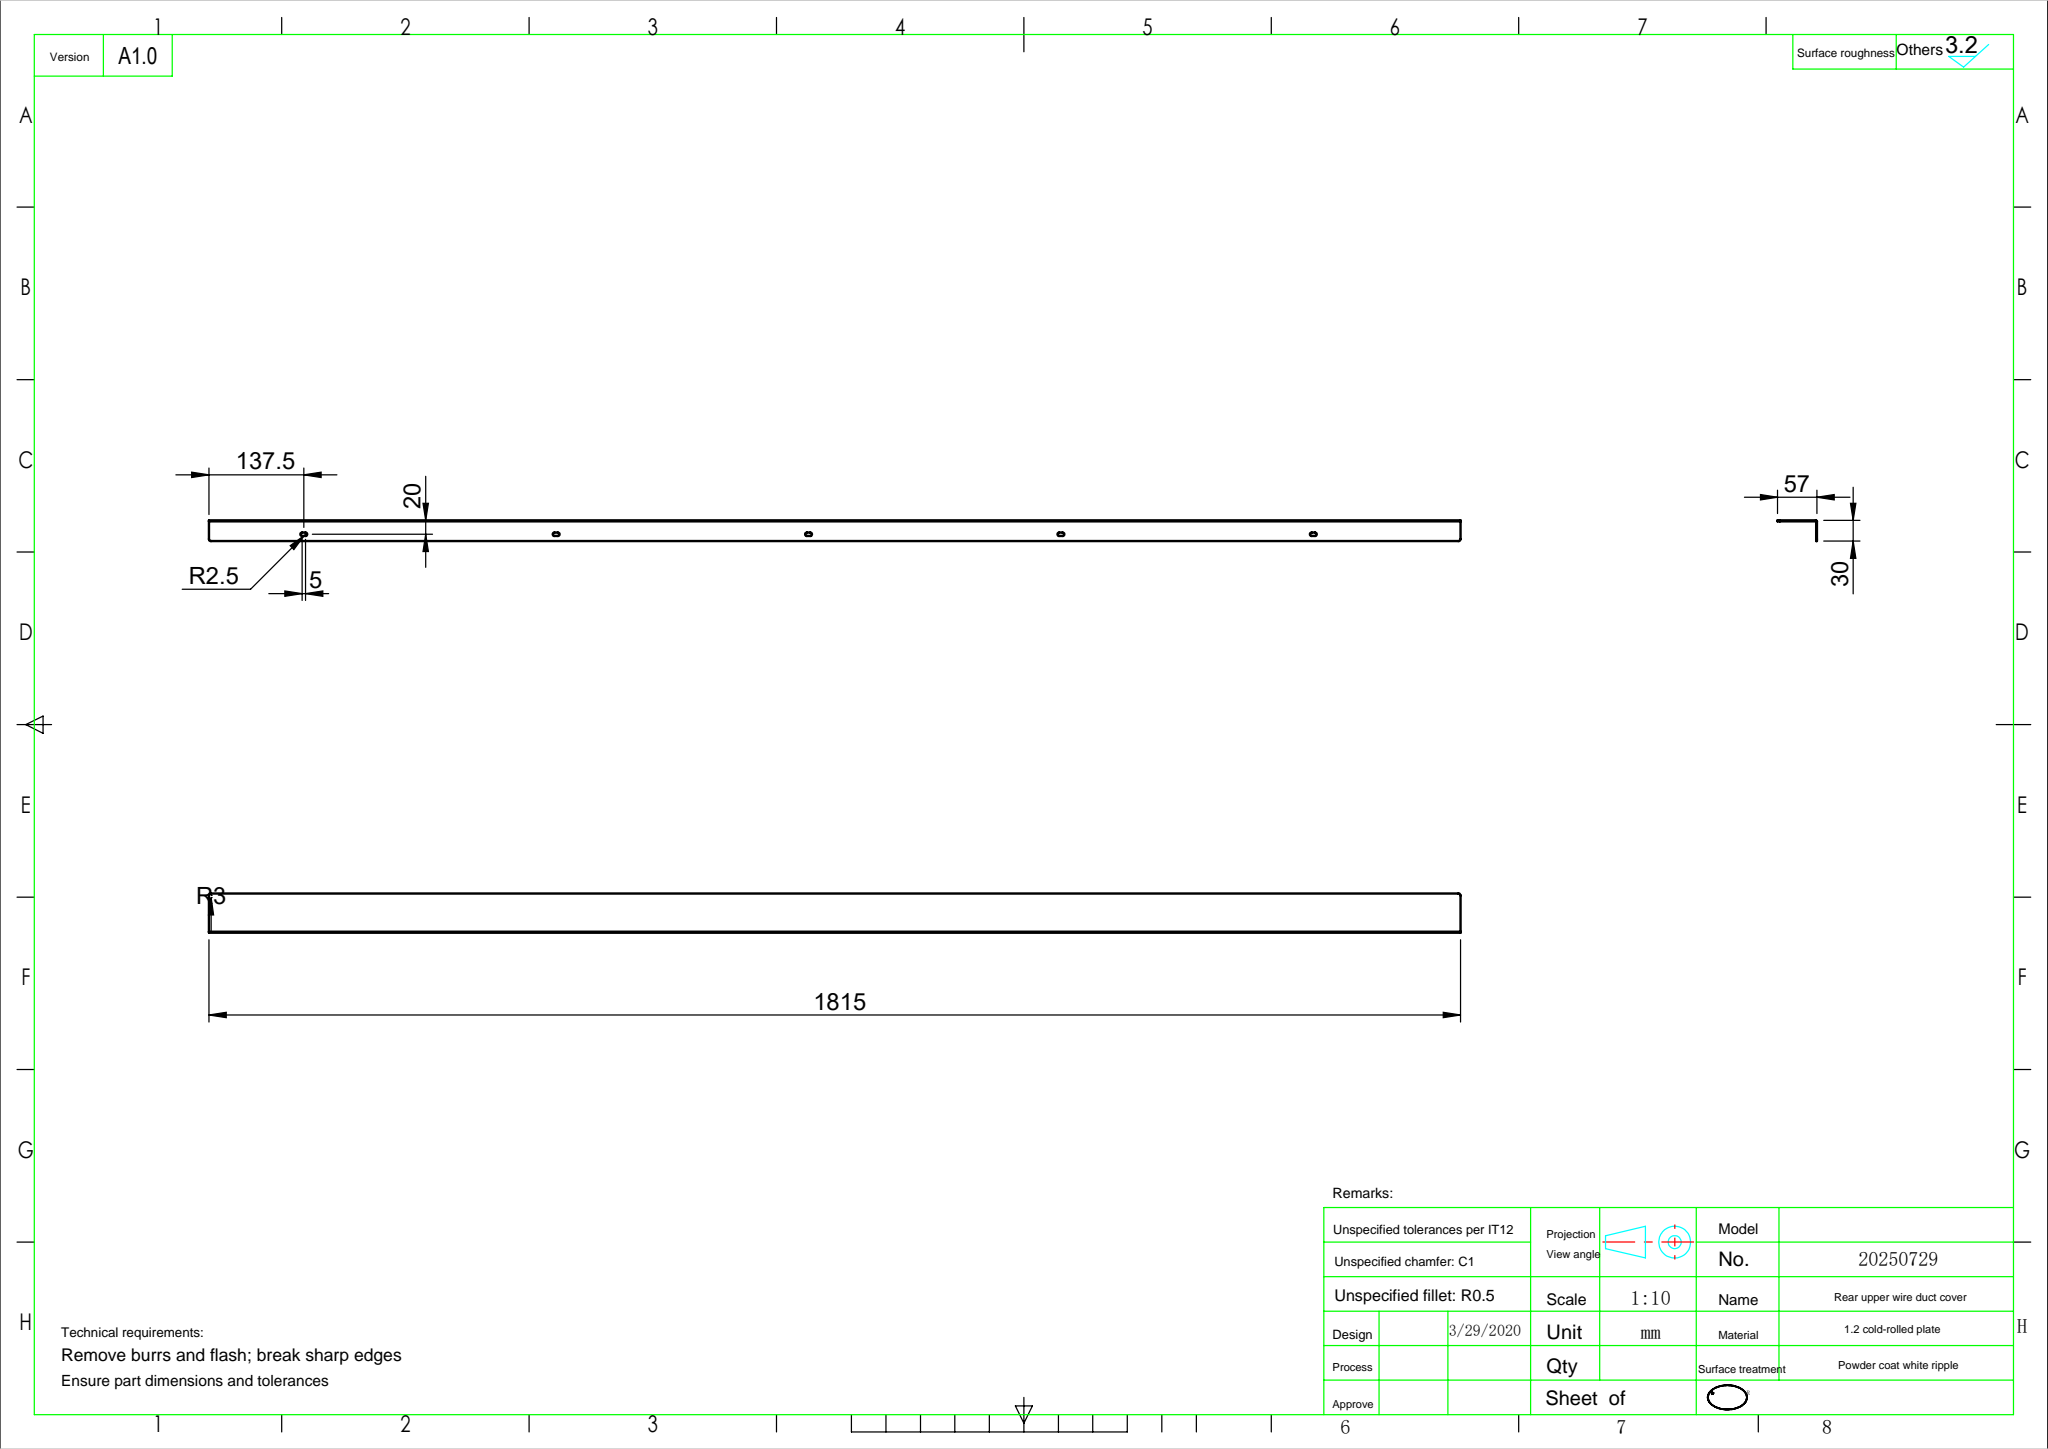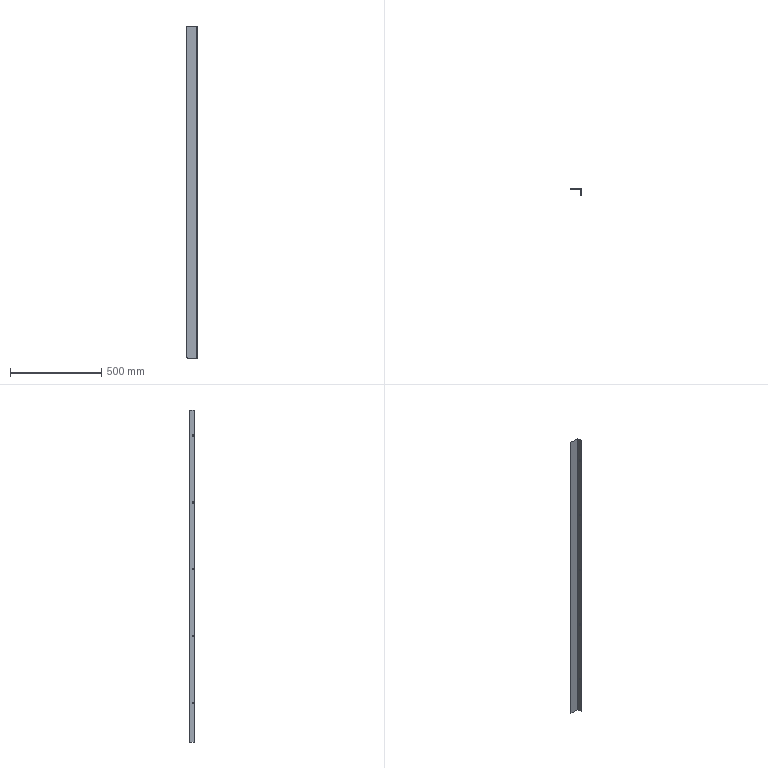Part | SolidWorks | features Fillet 1, FlatPattern 1, ICE 1, LPattern 1, SMBaseFlange 1, SheetMetal 1 | 1 solid | 43 faces | box 57 x 30 x 1815 mm | volume 185847 mm3 | plane 22 | cylinder 21 | commonest cylinder face diameters 5 x15 6 x4 0.4 x1 2.8 x1